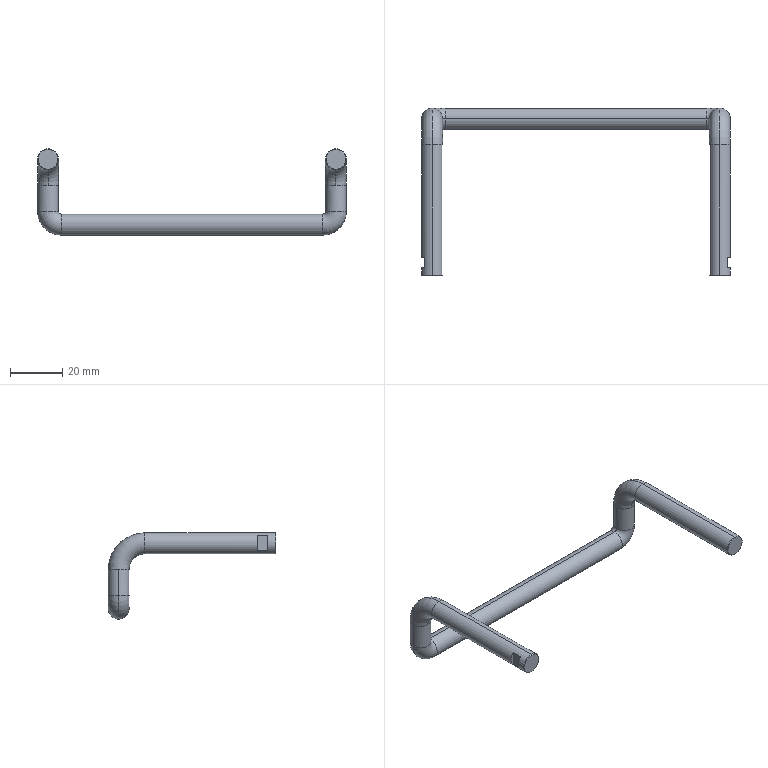Part | SolidWorks | features BaseBody 1 | 1 solid | 30 faces | box 118 x 64 x 33 mm | volume 13386 mm3 | cylinder 10 | torus 8 | plane 8 | cone 4 | commonest cylinder face diameters 8 x10
STEP:
#1=CARTESIAN_POINT('',(-55.,4.,15.));
#2=VERTEX_POINT('',#1);
#3=CARTESIAN_POINT('',(-51.,0.,15.));
#4=VERTEX_POINT('',#3);
#5=CARTESIAN_POINT('',(-55.,0.,15.));
#6=DIRECTION('',(0.,0.,-1.));
#7=DIRECTION('',(0.,-1.,0.));
#8=AXIS2_PLACEMENT_3D('',#5,#6,#7);
#9=CIRCLE('',#8,4.);
#10=EDGE_CURVE('',#2,#4,#9,.T.);
#11=ORIENTED_EDGE('',*,*,#10,.F.);
#12=CARTESIAN_POINT('',(-55.,-10.,29.));
#13=VERTEX_POINT('',#12);
#14=CARTESIAN_POINT('',(-55.,-10.,15.));
#15=DIRECTION('',(1.,0.,0.));
#16=DIRECTION('',(0.,0.,-1.));
#17=AXIS2_PLACEMENT_3D('',#14,#15,#16);
#18=CIRCLE('',#17,14.);
#19=EDGE_CURVE('',#2,#13,#18,.T.);
#20=ORIENTED_EDGE('',*,*,#19,.T.);
#21=CARTESIAN_POINT('',(-55.,-10.,21.));
#22=VERTEX_POINT('',#21);
#23=CARTESIAN_POINT('',(-55.,-10.,25.));
#24=DIRECTION('',(0.,1.,0.));
#25=DIRECTION('',(0.,0.,-1.));
#26=AXIS2_PLACEMENT_3D('',#23,#24,#25);
#27=CIRCLE('',#26,4.);
#28=EDGE_CURVE('',#13,#22,#27,.T.);
#29=ORIENTED_EDGE('',*,*,#28,.T.);
#30=CARTESIAN_POINT('',(-55.,-4.,15.));
#31=VERTEX_POINT('',#30);
#32=CARTESIAN_POINT('',(-55.,-10.,15.));
#33=DIRECTION('',(1.,0.,0.));
#34=DIRECTION('',(0.,0.,-1.));
#35=AXIS2_PLACEMENT_3D('',#32,#33,#34);
#36=CIRCLE('',#35,6.);
#37=EDGE_CURVE('',#31,#22,#36,.T.);
#38=ORIENTED_EDGE('',*,*,#37,.F.);
#39=CARTESIAN_POINT('',(-55.,0.,15.));
#40=DIRECTION('',(0.,0.,-1.));
#41=DIRECTION('',(0.,-1.,0.));
#42=AXIS2_PLACEMENT_3D('',#39,#40,#41);
#43=CIRCLE('',#42,4.);
#44=EDGE_CURVE('',#4,#31,#43,.T.);
#45=ORIENTED_EDGE('',*,*,#44,.F.);
#46=EDGE_LOOP('',(#11,#20,#29,#38,#45));
#47=FACE_OUTER_BOUND('',#46,.T.);
#48=CARTESIAN_POINT('',(-55.,-10.,15.));
#49=DIRECTION('',(1.,0.,0.));
#50=DIRECTION('',(0.,0.,-1.));
#51=AXIS2_PLACEMENT_3D('',#48,#49,#50);
#52=TOROIDAL_SURFACE('',#51,10.,4.);
#53=ADVANCED_FACE('',(#47),#52,.T.);
#54=CARTESIAN_POINT('',(-50.,0.,-4.));
#55=VERTEX_POINT('',#54);
#56=CARTESIAN_POINT('',(-50.,0.,4.));
#57=VERTEX_POINT('',#56);
#58=CARTESIAN_POINT('',(-50.,0.,0.));
#59=DIRECTION('',(1.,0.,0.));
#60=DIRECTION('',(0.,-1.,0.));
#61=AXIS2_PLACEMENT_3D('',#58,#59,#60);
#62=CIRCLE('',#61,4.);
#63=EDGE_CURVE('',#55,#57,#62,.T.);
#64=ORIENTED_EDGE('',*,*,#63,.F.);
#65=CARTESIAN_POINT('',(-59.,0.,5.));
#66=VERTEX_POINT('',#65);
#67=CARTESIAN_POINT('',(-50.,0.,5.));
#68=DIRECTION('',(0.,1.,0.));
#69=DIRECTION('',(0.,0.,1.));
#70=AXIS2_PLACEMENT_3D('',#67,#68,#69);
#71=CIRCLE('',#70,9.);
#72=EDGE_CURVE('',#55,#66,#71,.T.);
#73=ORIENTED_EDGE('',*,*,#72,.T.);
#74=CARTESIAN_POINT('',(-51.,0.,5.));
#75=VERTEX_POINT('',#74);
#76=CARTESIAN_POINT('',(-55.,0.,5.));
#77=DIRECTION('',(0.,0.,-1.));
#78=DIRECTION('',(0.,-1.,0.));
#79=AXIS2_PLACEMENT_3D('',#76,#77,#78);
#80=CIRCLE('',#79,4.);
#81=EDGE_CURVE('',#66,#75,#80,.T.);
#82=ORIENTED_EDGE('',*,*,#81,.T.);
#83=CARTESIAN_POINT('',(-50.,0.,5.));
#84=DIRECTION('',(0.,1.,0.));
#85=DIRECTION('',(0.,0.,1.));
#86=AXIS2_PLACEMENT_3D('',#83,#84,#85);
#87=CIRCLE('',#86,1.);
#88=EDGE_CURVE('',#57,#75,#87,.T.);
#89=ORIENTED_EDGE('',*,*,#88,.F.);
#90=EDGE_LOOP('',(#64,#73,#82,#89));
#91=FACE_OUTER_BOUND('',#90,.T.);
#92=CARTESIAN_POINT('',(-50.,0.,5.));
#93=DIRECTION('',(0.,1.,0.));
#94=DIRECTION('',(0.,0.,1.));
#95=AXIS2_PLACEMENT_3D('',#92,#93,#94);
#96=TOROIDAL_SURFACE('',#95,5.,4.);
#97=ADVANCED_FACE('',(#91),#96,.T.);
#98=CARTESIAN_POINT('',(59.,0.,5.));
#99=VERTEX_POINT('',#98);
#100=CARTESIAN_POINT('',(51.,0.,5.));
#101=VERTEX_POINT('',#100);
#102=CARTESIAN_POINT('',(55.,0.,5.));
#103=DIRECTION('',(0.,0.,1.));
#104=DIRECTION('',(0.,-1.,0.));
#105=AXIS2_PLACEMENT_3D('',#102,#103,#104);
#106=CIRCLE('',#105,4.);
#107=EDGE_CURVE('',#99,#101,#106,.T.);
#108=ORIENTED_EDGE('',*,*,#107,.F.);
#109=CARTESIAN_POINT('',(50.,0.,-4.));
#110=VERTEX_POINT('',#109);
#111=CARTESIAN_POINT('',(50.,0.,5.));
#112=DIRECTION('',(0.,1.,0.));
#113=DIRECTION('',(0.,0.,1.));
#114=AXIS2_PLACEMENT_3D('',#111,#112,#113);
#115=CIRCLE('',#114,9.);
#116=EDGE_CURVE('',#99,#110,#115,.T.);
#117=ORIENTED_EDGE('',*,*,#116,.T.);
#118=CARTESIAN_POINT('',(50.,0.,4.));
#119=VERTEX_POINT('',#118);
#120=CARTESIAN_POINT('',(50.,0.,0.));
#121=DIRECTION('',(1.,0.,0.));
#122=DIRECTION('',(0.,-1.,0.));
#123=AXIS2_PLACEMENT_3D('',#120,#121,#122);
#124=CIRCLE('',#123,4.);
#125=EDGE_CURVE('',#110,#119,#124,.T.);
#126=ORIENTED_EDGE('',*,*,#125,.T.);
#127=CARTESIAN_POINT('',(50.,0.,5.));
#128=DIRECTION('',(0.,1.,0.));
#129=DIRECTION('',(0.,0.,1.));
#130=AXIS2_PLACEMENT_3D('',#127,#128,#129);
#131=CIRCLE('',#130,1.);
#132=EDGE_CURVE('',#101,#119,#131,.T.);
#133=ORIENTED_EDGE('',*,*,#132,.F.);
#134=EDGE_LOOP('',(#108,#117,#126,#133));
#135=FACE_OUTER_BOUND('',#134,.T.);
#136=CARTESIAN_POINT('',(50.,0.,5.));
#137=DIRECTION('',(0.,1.,0.));
#138=DIRECTION('',(0.,0.,1.));
#139=AXIS2_PLACEMENT_3D('',#136,#137,#138);
#140=TOROIDAL_SURFACE('',#139,5.,4.);
#141=ADVANCED_FACE('',(#135),#140,.T.);
#142=CARTESIAN_POINT('',(55.,-10.,29.));
#143=VERTEX_POINT('',#142);
#144=CARTESIAN_POINT('',(55.,-10.,21.));
#145=VERTEX_POINT('',#144);
#146=CARTESIAN_POINT('',(55.,-10.,25.));
#147=DIRECTION('',(0.,-1.,0.));
#148=DIRECTION('',(0.,0.,-1.));
#149=AXIS2_PLACEMENT_3D('',#146,#147,#148);
#150=CIRCLE('',#149,4.);
#151=EDGE_CURVE('',#143,#145,#150,.T.);
#152=ORIENTED_EDGE('',*,*,#151,.F.);
#153=CARTESIAN_POINT('',(55.,4.,15.));
#154=VERTEX_POINT('',#153);
#155=CARTESIAN_POINT('',(55.,-10.,15.));
#156=DIRECTION('',(-1.,0.,0.));
#157=DIRECTION('',(0.,0.,1.));
#158=AXIS2_PLACEMENT_3D('',#155,#156,#157);
#159=CIRCLE('',#158,14.);
#160=EDGE_CURVE('',#143,#154,#159,.T.);
#161=ORIENTED_EDGE('',*,*,#160,.T.);
#162=CARTESIAN_POINT('',(51.,0.,15.));
#163=VERTEX_POINT('',#162);
#164=CARTESIAN_POINT('',(55.,0.,15.));
#165=DIRECTION('',(0.,0.,1.));
#166=DIRECTION('',(0.,-1.,0.));
#167=AXIS2_PLACEMENT_3D('',#164,#165,#166);
#168=CIRCLE('',#167,4.);
#169=EDGE_CURVE('',#154,#163,#168,.T.);
#170=ORIENTED_EDGE('',*,*,#169,.T.);
#171=CARTESIAN_POINT('',(55.,-4.,15.));
#172=VERTEX_POINT('',#171);
#173=CARTESIAN_POINT('',(55.,0.,15.));
#174=DIRECTION('',(0.,0.,1.));
#175=DIRECTION('',(0.,-1.,0.));
#176=AXIS2_PLACEMENT_3D('',#173,#174,#175);
#177=CIRCLE('',#176,4.);
#178=EDGE_CURVE('',#163,#172,#177,.T.);
#179=ORIENTED_EDGE('',*,*,#178,.T.);
#180=CARTESIAN_POINT('',(55.,-10.,15.));
#181=DIRECTION('',(-1.,0.,0.));
#182=DIRECTION('',(0.,0.,1.));
#183=AXIS2_PLACEMENT_3D('',#180,#181,#182);
#184=CIRCLE('',#183,6.);
#185=EDGE_CURVE('',#145,#172,#184,.T.);
#186=ORIENTED_EDGE('',*,*,#185,.F.);
#187=EDGE_LOOP('',(#152,#161,#170,#179,#186));
#188=FACE_OUTER_BOUND('',#187,.T.);
#189=CARTESIAN_POINT('',(55.,-10.,15.));
#190=DIRECTION('',(-1.,0.,0.));
#191=DIRECTION('',(0.,0.,1.));
#192=AXIS2_PLACEMENT_3D('',#189,#190,#191);
#193=TOROIDAL_SURFACE('',#192,10.,4.);
#194=ADVANCED_FACE('',(#188),#193,.T.);
#195=CARTESIAN_POINT('',(-55.,-60.,21.2));
#196=VERTEX_POINT('',#195);
#197=CARTESIAN_POINT('',(-55.,-60.,28.8));
#198=VERTEX_POINT('',#197);
#199=CARTESIAN_POINT('',(-55.,-60.,25.));
#200=DIRECTION('',(0.,-1.,0.));
#201=DIRECTION('',(0.,0.,1.));
#202=AXIS2_PLACEMENT_3D('',#199,#200,#201);
#203=CIRCLE('',#202,3.8);
#204=EDGE_CURVE('',#196,#198,#203,.T.);
#205=ORIENTED_EDGE('',*,*,#204,.F.);
#206=CARTESIAN_POINT('',(-55.,-59.8,21.));
#207=VERTEX_POINT('',#206);
#208=CARTESIAN_POINT('',(-55.,-59.8,21.));
#209=DIRECTION('',(0.,0.7071,-0.7071));
#210=VECTOR('',#209,1000.);
#211=LINE('',#208,#210);
#212=EDGE_CURVE('',#196,#207,#211,.T.);
#213=ORIENTED_EDGE('',*,*,#212,.T.);
#214=CARTESIAN_POINT('',(-55.,-59.8,29.));
#215=VERTEX_POINT('',#214);
#216=CARTESIAN_POINT('',(-55.,-59.8,25.));
#217=DIRECTION('',(0.,1.,0.));
#218=DIRECTION('',(0.,0.,1.));
#219=AXIS2_PLACEMENT_3D('',#216,#217,#218);
#220=CIRCLE('',#219,4.);
#221=EDGE_CURVE('',#215,#207,#220,.T.);
#222=ORIENTED_EDGE('',*,*,#221,.F.);
#223=CARTESIAN_POINT('',(-55.,-59.8,29.));
#224=DIRECTION('',(0.,0.7071,0.7071));
#225=VECTOR('',#224,1000.);
#226=LINE('',#223,#225);
#227=EDGE_CURVE('',#198,#215,#226,.T.);
#228=ORIENTED_EDGE('',*,*,#227,.F.);
#229=EDGE_LOOP('',(#205,#213,#222,#228));
#230=FACE_OUTER_BOUND('',#229,.T.);
#231=CARTESIAN_POINT('',(-55.,-59.8,25.));
#232=DIRECTION('',(0.,1.,0.));
#233=DIRECTION('',(0.,0.,1.));
#234=AXIS2_PLACEMENT_3D('',#231,#232,#233);
#235=CONICAL_SURFACE('',#234,4.,0.7854);
#236=ADVANCED_FACE('',(#230),#235,.T.);
#237=CARTESIAN_POINT('',(55.,-60.,21.2));
#238=VERTEX_POINT('',#237);
#239=CARTESIAN_POINT('',(55.,-60.,28.8));
#240=VERTEX_POINT('',#239);
#241=CARTESIAN_POINT('',(55.,-60.,25.));
#242=DIRECTION('',(0.,-1.,0.));
#243=DIRECTION('',(0.,0.,-1.));
#244=AXIS2_PLACEMENT_3D('',#241,#242,#243);
#245=CIRCLE('',#244,3.8);
#246=EDGE_CURVE('',#238,#240,#245,.T.);
#247=ORIENTED_EDGE('',*,*,#246,.F.);
#248=CARTESIAN_POINT('',(55.,-59.8,21.));
#249=VERTEX_POINT('',#248);
#250=CARTESIAN_POINT('',(55.,-60.,21.2));
#251=DIRECTION('',(0.,0.7071,-0.7071));
#252=VECTOR('',#251,1000.);
#253=LINE('',#250,#252);
#254=EDGE_CURVE('',#238,#249,#253,.T.);
#255=ORIENTED_EDGE('',*,*,#254,.T.);
#256=CARTESIAN_POINT('',(55.,-59.8,29.));
#257=VERTEX_POINT('',#256);
#258=CARTESIAN_POINT('',(55.,-59.8,25.));
#259=DIRECTION('',(0.,1.,0.));
#260=DIRECTION('',(0.,0.,-1.));
#261=AXIS2_PLACEMENT_3D('',#258,#259,#260);
#262=CIRCLE('',#261,4.);
#263=EDGE_CURVE('',#257,#249,#262,.T.);
#264=ORIENTED_EDGE('',*,*,#263,.F.);
#265=CARTESIAN_POINT('',(55.,-60.,28.8));
#266=DIRECTION('',(0.,0.7071,0.7071));
#267=VECTOR('',#266,1000.);
#268=LINE('',#265,#267);
#269=EDGE_CURVE('',#240,#257,#268,.T.);
#270=ORIENTED_EDGE('',*,*,#269,.F.);
#271=EDGE_LOOP('',(#247,#255,#264,#270));
#272=FACE_OUTER_BOUND('',#271,.T.);
#273=CARTESIAN_POINT('',(55.,-60.,25.));
#274=DIRECTION('',(0.,1.,0.));
#275=DIRECTION('',(0.,0.,1.));
#276=AXIS2_PLACEMENT_3D('',#273,#274,#275);
#277=CONICAL_SURFACE('',#276,3.8,0.7854);
#278=ADVANCED_FACE('',(#272),#277,.T.);
#279=ORIENTED_EDGE('',*,*,#28,.F.);
#280=CARTESIAN_POINT('',(-55.,-10.,29.));
#281=DIRECTION('',(0.,-1.,0.));
#282=VECTOR('',#281,1000.);
#283=LINE('',#280,#282);
#284=EDGE_CURVE('',#13,#215,#283,.T.);
#285=ORIENTED_EDGE('',*,*,#284,.T.);
#286=ORIENTED_EDGE('',*,*,#221,.T.);
#287=CARTESIAN_POINT('',(-55.,-10.,21.));
#288=DIRECTION('',(0.,-1.,0.));
#289=VECTOR('',#288,1000.);
#290=LINE('',#287,#289);
#291=EDGE_CURVE('',#22,#207,#290,.T.);
#292=ORIENTED_EDGE('',*,*,#291,.F.);
#293=EDGE_LOOP('',(#279,#285,#286,#292));
#294=FACE_OUTER_BOUND('',#293,.T.);
#295=CARTESIAN_POINT('',(-55.,-10.,25.));
#296=DIRECTION('',(0.,-1.,0.));
#297=DIRECTION('',(0.,0.,-1.));
#298=AXIS2_PLACEMENT_3D('',#295,#296,#297);
#299=CYLINDRICAL_SURFACE('',#298,4.);
#300=ADVANCED_FACE('',(#294),#299,.T.);
#301=ORIENTED_EDGE('',*,*,#81,.F.);
#302=CARTESIAN_POINT('',(-59.,0.,15.));
#303=VERTEX_POINT('',#302);
#304=CARTESIAN_POINT('',(-59.,0.,5.));
#305=DIRECTION('',(0.,0.,1.));
#306=VECTOR('',#305,1000.);
#307=LINE('',#304,#306);
#308=EDGE_CURVE('',#66,#303,#307,.T.);
#309=ORIENTED_EDGE('',*,*,#308,.T.);
#310=CARTESIAN_POINT('',(-55.,0.,15.));
#311=DIRECTION('',(0.,0.,-1.));
#312=DIRECTION('',(0.,-1.,0.));
#313=AXIS2_PLACEMENT_3D('',#310,#311,#312);
#314=CIRCLE('',#313,4.);
#315=EDGE_CURVE('',#303,#2,#314,.T.);
#316=ORIENTED_EDGE('',*,*,#315,.T.);
#317=ORIENTED_EDGE('',*,*,#10,.T.);
#318=CARTESIAN_POINT('',(-51.,0.,5.));
#319=DIRECTION('',(0.,0.,1.));
#320=VECTOR('',#319,1000.);
#321=LINE('',#318,#320);
#322=EDGE_CURVE('',#75,#4,#321,.T.);
#323=ORIENTED_EDGE('',*,*,#322,.F.);
#324=EDGE_LOOP('',(#301,#309,#316,#317,#323));
#325=FACE_OUTER_BOUND('',#324,.T.);
#326=CARTESIAN_POINT('',(-55.,0.,5.));
#327=DIRECTION('',(0.,0.,1.));
#328=DIRECTION('',(1.,0.,0.));
#329=AXIS2_PLACEMENT_3D('',#326,#327,#328);
#330=CYLINDRICAL_SURFACE('',#329,4.);
#331=ADVANCED_FACE('',(#325),#330,.T.);
#332=ORIENTED_EDGE('',*,*,#125,.F.);
#333=CARTESIAN_POINT('',(50.,0.,-4.));
#334=DIRECTION('',(-1.,0.,0.));
#335=VECTOR('',#334,1000.);
#336=LINE('',#333,#335);
#337=EDGE_CURVE('',#110,#55,#336,.T.);
#338=ORIENTED_EDGE('',*,*,#337,.T.);
#339=ORIENTED_EDGE('',*,*,#63,.T.);
#340=CARTESIAN_POINT('',(50.,0.,4.));
#341=DIRECTION('',(-1.,0.,0.));
#342=VECTOR('',#341,1000.);
#343=LINE('',#340,#342);
#344=EDGE_CURVE('',#119,#57,#343,.T.);
#345=ORIENTED_EDGE('',*,*,#344,.F.);
#346=EDGE_LOOP('',(#332,#338,#339,#345));
#347=FACE_OUTER_BOUND('',#346,.T.);
#348=CARTESIAN_POINT('',(50.,0.,0.));
#349=DIRECTION('',(-1.,0.,0.));
#350=DIRECTION('',(0.,0.,1.));
#351=AXIS2_PLACEMENT_3D('',#348,#349,#350);
#352=CYLINDRICAL_SURFACE('',#351,4.);
#353=ADVANCED_FACE('',(#347),#352,.T.);
#354=CARTESIAN_POINT('',(59.,0.,15.));
#355=VERTEX_POINT('',#354);
#356=CARTESIAN_POINT('',(55.,0.,15.));
#357=DIRECTION('',(0.,0.,1.));
#358=DIRECTION('',(0.,-1.,0.));
#359=AXIS2_PLACEMENT_3D('',#356,#357,#358);
#360=CIRCLE('',#359,4.);
#361=EDGE_CURVE('',#355,#154,#360,.T.);
#362=ORIENTED_EDGE('',*,*,#361,.F.);
#363=CARTESIAN_POINT('',(59.,0.,15.));
#364=DIRECTION('',(0.,0.,-1.));
#365=VECTOR('',#364,1000.);
#366=LINE('',#363,#365);
#367=EDGE_CURVE('',#355,#99,#366,.T.);
#368=ORIENTED_EDGE('',*,*,#367,.T.);
#369=ORIENTED_EDGE('',*,*,#107,.T.);
#370=CARTESIAN_POINT('',(51.,0.,15.));
#371=DIRECTION('',(0.,0.,-1.));
#372=VECTOR('',#371,1000.);
#373=LINE('',#370,#372);
#374=EDGE_CURVE('',#163,#101,#373,.T.);
#375=ORIENTED_EDGE('',*,*,#374,.F.);
#376=ORIENTED_EDGE('',*,*,#169,.F.);
#377=EDGE_LOOP('',(#362,#368,#369,#375,#376));
#378=FACE_OUTER_BOUND('',#377,.T.);
#379=CARTESIAN_POINT('',(55.,0.,15.));
#380=DIRECTION('',(0.,0.,-1.));
#381=DIRECTION('',(-1.,0.,0.));
#382=AXIS2_PLACEMENT_3D('',#379,#380,#381);
#383=CYLINDRICAL_SURFACE('',#382,4.);
#384=ADVANCED_FACE('',(#378),#383,.T.);
#385=CARTESIAN_POINT('',(57.75,-53.,22.095));
#386=VERTEX_POINT('',#385);
#387=CARTESIAN_POINT('',(57.75,-57.,22.095));
#388=VERTEX_POINT('',#387);
#389=CARTESIAN_POINT('',(57.75,-60.,22.095));
#390=DIRECTION('',(0.,-1.,0.));
#391=VECTOR('',#390,1000.);
#392=LINE('',#389,#391);
#393=EDGE_CURVE('',#386,#388,#392,.T.);
#394=ORIENTED_EDGE('',*,*,#393,.T.);
#395=CARTESIAN_POINT('',(57.75,-57.,27.905));
#396=VERTEX_POINT('',#395);
#397=CARTESIAN_POINT('',(55.,-57.,25.));
#398=DIRECTION('',(0.,-1.,0.));
#399=DIRECTION('',(0.,0.,-1.));
#400=AXIS2_PLACEMENT_3D('',#397,#398,#399);
#401=CIRCLE('',#400,4.);
#402=EDGE_CURVE('',#388,#396,#401,.T.);
#403=ORIENTED_EDGE('',*,*,#402,.T.);
#404=CARTESIAN_POINT('',(57.75,-53.,27.905));
#405=VERTEX_POINT('',#404);
#406=CARTESIAN_POINT('',(57.75,-60.,27.905));
#407=DIRECTION('',(0.,1.,0.));
#408=VECTOR('',#407,1000.);
#409=LINE('',#406,#408);
#410=EDGE_CURVE('',#396,#405,#409,.T.);
#411=ORIENTED_EDGE('',*,*,#410,.T.);
#412=CARTESIAN_POINT('',(55.,-53.,25.));
#413=DIRECTION('',(0.,1.,0.));
#414=DIRECTION('',(0.,0.,1.));
#415=AXIS2_PLACEMENT_3D('',#412,#413,#414);
#416=CIRCLE('',#415,4.);
#417=EDGE_CURVE('',#405,#386,#416,.T.);
#418=ORIENTED_EDGE('',*,*,#417,.T.);
#419=EDGE_LOOP('',(#394,#403,#411,#418));
#420=FACE_BOUND('',#419,.T.);
#421=ORIENTED_EDGE('',*,*,#263,.T.);
#422=CARTESIAN_POINT('',(55.,-60.,21.));
#423=DIRECTION('',(0.,1.,0.));
#424=VECTOR('',#423,1000.);
#425=LINE('',#422,#424);
#426=EDGE_CURVE('',#249,#145,#425,.T.);
#427=ORIENTED_EDGE('',*,*,#426,.T.);
#428=CARTESIAN_POINT('',(55.,-10.,25.));
#429=DIRECTION('',(0.,-1.,0.));
#430=DIRECTION('',(0.,0.,-1.));
#431=AXIS2_PLACEMENT_3D('',#428,#429,#430);
#432=CIRCLE('',#431,4.);
#433=EDGE_CURVE('',#145,#143,#432,.T.);
#434=ORIENTED_EDGE('',*,*,#433,.T.);
#435=CARTESIAN_POINT('',(55.,-60.,29.));
#436=DIRECTION('',(0.,1.,0.));
#437=VECTOR('',#436,1000.);
#438=LINE('',#435,#437);
#439=EDGE_CURVE('',#257,#143,#438,.T.);
#440=ORIENTED_EDGE('',*,*,#439,.F.);
#441=EDGE_LOOP('',(#421,#427,#434,#440));
#442=FACE_OUTER_BOUND('',#441,.T.);
#443=CARTESIAN_POINT('',(55.,-60.,25.));
#444=DIRECTION('',(0.,1.,0.));
#445=DIRECTION('',(0.,0.,1.));
#446=AXIS2_PLACEMENT_3D('',#443,#444,#445);
#447=CYLINDRICAL_SURFACE('',#446,4.);
#448=ADVANCED_FACE('',(#420,#442),#447,.T.);
#449=CARTESIAN_POINT('',(57.75,-53.,-4.));
#450=DIRECTION('',(0.,0.,1.));
#451=VECTOR('',#450,1000.);
#452=LINE('',#449,#451);
#453=EDGE_CURVE('',#386,#405,#452,.T.);
#454=ORIENTED_EDGE('',*,*,#453,.F.);
#455=ORIENTED_EDGE('',*,*,#417,.F.);
#456=EDGE_LOOP('',(#454,#455));
#457=FACE_OUTER_BOUND('',#456,.T.);
#458=CARTESIAN_POINT('',(57.75,-53.,-4.));
#459=DIRECTION('',(0.,1.,0.));
#460=DIRECTION('',(1.,0.,0.));
#461=AXIS2_PLACEMENT_3D('',#458,#459,#460);
#462=PLANE('',#461);
#463=ADVANCED_FACE('',(#457),#462,.F.);
#464=CARTESIAN_POINT('',(57.75,-57.,-4.));
#465=DIRECTION('',(0.,0.,1.));
#466=VECTOR('',#465,1000.);
#467=LINE('',#464,#466);
#468=EDGE_CURVE('',#388,#396,#467,.T.);
#469=ORIENTED_EDGE('',*,*,#468,.F.);
#470=ORIENTED_EDGE('',*,*,#393,.F.);
#471=ORIENTED_EDGE('',*,*,#453,.T.);
#472=ORIENTED_EDGE('',*,*,#410,.F.);
#473=EDGE_LOOP('',(#469,#470,#471,#472));
#474=FACE_OUTER_BOUND('',#473,.T.);
#475=CARTESIAN_POINT('',(57.75,-57.,-4.));
#476=DIRECTION('',(-1.,0.,0.));
#477=DIRECTION('',(0.,1.,0.));
#478=AXIS2_PLACEMENT_3D('',#475,#476,#477);
#479=PLANE('',#478);
#480=ADVANCED_FACE('',(#474),#479,.F.);
#481=ORIENTED_EDGE('',*,*,#468,.T.);
#482=ORIENTED_EDGE('',*,*,#402,.F.);
#483=EDGE_LOOP('',(#481,#482));
#484=FACE_OUTER_BOUND('',#483,.T.);
#485=CARTESIAN_POINT('',(57.75,-57.,-4.));
#486=DIRECTION('',(0.,-1.,0.));
#487=DIRECTION('',(0.,0.,-1.));
#488=AXIS2_PLACEMENT_3D('',#485,#486,#487);
#489=PLANE('',#488);
#490=ADVANCED_FACE('',(#484),#489,.F.);
#491=CARTESIAN_POINT('',(-57.75,-53.,22.095));
#492=VERTEX_POINT('',#491);
#493=CARTESIAN_POINT('',(-57.75,-53.,27.905));
#494=VERTEX_POINT('',#493);
#495=CARTESIAN_POINT('',(-57.75,-53.,-4.));
#496=DIRECTION('',(0.,0.,1.));
#497=VECTOR('',#496,1000.);
#498=LINE('',#495,#497);
#499=EDGE_CURVE('',#492,#494,#498,.T.);
#500=ORIENTED_EDGE('',*,*,#499,.T.);
#501=CARTESIAN_POINT('',(-55.,-53.,25.));
#502=DIRECTION('',(0.,1.,0.));
#503=DIRECTION('',(-1.,0.,0.));
#504=AXIS2_PLACEMENT_3D('',#501,#502,#503);
#505=CIRCLE('',#504,4.);
#506=EDGE_CURVE('',#492,#494,#505,.T.);
#507=ORIENTED_EDGE('',*,*,#506,.F.);
#508=EDGE_LOOP('',(#500,#507));
#509=FACE_OUTER_BOUND('',#508,.T.);
#510=CARTESIAN_POINT('',(-60.25,-53.,-4.));
#511=DIRECTION('',(0.,1.,0.));
#512=DIRECTION('',(1.,0.,0.));
#513=AXIS2_PLACEMENT_3D('',#510,#511,#512);
#514=PLANE('',#513);
#515=ADVANCED_FACE('',(#509),#514,.F.);
#516=CARTESIAN_POINT('',(-57.75,-57.,22.095));
#517=VERTEX_POINT('',#516);
#518=CARTESIAN_POINT('',(-57.75,-57.,27.905));
#519=VERTEX_POINT('',#518);
#520=CARTESIAN_POINT('',(-57.75,-57.,-4.));
#521=DIRECTION('',(0.,0.,1.));
#522=VECTOR('',#521,1000.);
#523=LINE('',#520,#522);
#524=EDGE_CURVE('',#517,#519,#523,.T.);
#525=ORIENTED_EDGE('',*,*,#524,.F.);
#526=CARTESIAN_POINT('',(-55.,-57.,25.));
#527=DIRECTION('',(0.,-1.,0.));
#528=DIRECTION('',(0.,0.,-1.));
#529=AXIS2_PLACEMENT_3D('',#526,#527,#528);
#530=CIRCLE('',#529,4.);
#531=EDGE_CURVE('',#519,#517,#530,.T.);
#532=ORIENTED_EDGE('',*,*,#531,.F.);
#533=EDGE_LOOP('',(#525,#532));
#534=FACE_OUTER_BOUND('',#533,.T.);
#535=CARTESIAN_POINT('',(-60.25,-57.,-4.));
#536=DIRECTION('',(0.,-1.,0.));
#537=DIRECTION('',(0.,0.,-1.));
#538=AXIS2_PLACEMENT_3D('',#535,#536,#537);
#539=PLANE('',#538);
#540=ADVANCED_FACE('',(#534),#539,.F.);
#541=ORIENTED_EDGE('',*,*,#499,.F.);
#542=CARTESIAN_POINT('',(-57.75,-10.,22.095));
#543=DIRECTION('',(0.,1.,0.));
#544=VECTOR('',#543,1000.);
#545=LINE('',#542,#544);
#546=EDGE_CURVE('',#517,#492,#545,.T.);
#547=ORIENTED_EDGE('',*,*,#546,.F.);
#548=ORIENTED_EDGE('',*,*,#524,.T.);
#549=CARTESIAN_POINT('',(-57.75,-10.,27.905));
#550=DIRECTION('',(0.,-1.,0.));
#551=VECTOR('',#550,1000.);
#552=LINE('',#549,#551);
#553=EDGE_CURVE('',#494,#519,#552,.T.);
#554=ORIENTED_EDGE('',*,*,#553,.F.);
#555=EDGE_LOOP('',(#541,#547,#548,#554));
#556=FACE_OUTER_BOUND('',#555,.T.);
#557=CARTESIAN_POINT('',(-57.75,-57.,-4.));
#558=DIRECTION('',(1.,0.,0.));
#559=DIRECTION('',(0.,1.,0.));
#560=AXIS2_PLACEMENT_3D('',#557,#558,#559);
#561=PLANE('',#560);
#562=ADVANCED_FACE('',(#556),#561,.F.);
#563=CARTESIAN_POINT('',(55.,-60.,25.));
#564=DIRECTION('',(0.,-1.,0.));
#565=DIRECTION('',(0.,0.,-1.));
#566=AXIS2_PLACEMENT_3D('',#563,#564,#565);
#567=CIRCLE('',#566,3.8);
#568=EDGE_CURVE('',#240,#238,#567,.T.);
#569=ORIENTED_EDGE('',*,*,#568,.T.);
#570=ORIENTED_EDGE('',*,*,#246,.T.);
#571=EDGE_LOOP('',(#569,#570));
#572=FACE_OUTER_BOUND('',#571,.T.);
#573=CARTESIAN_POINT('',(55.,-60.,25.));
#574=DIRECTION('',(0.,-1.,0.));
#575=DIRECTION('',(0.,0.,-1.));
#576=AXIS2_PLACEMENT_3D('',#573,#574,#575);
#577=PLANE('',#576);
#578=ADVANCED_FACE('',(#572),#577,.T.);
#579=CARTESIAN_POINT('',(-55.,-60.,25.));
#580=DIRECTION('',(0.,-1.,0.));
#581=DIRECTION('',(0.,0.,1.));
#582=AXIS2_PLACEMENT_3D('',#579,#580,#581);
#583=CIRCLE('',#582,3.8);
#584=EDGE_CURVE('',#198,#196,#583,.T.);
#585=ORIENTED_EDGE('',*,*,#584,.T.);
#586=ORIENTED_EDGE('',*,*,#204,.T.);
#587=EDGE_LOOP('',(#585,#586));
#588=FACE_OUTER_BOUND('',#587,.T.);
#589=CARTESIAN_POINT('',(-55.,-60.,25.));
#590=DIRECTION('',(0.,1.,0.));
#591=DIRECTION('',(1.,0.,0.));
#592=AXIS2_PLACEMENT_3D('',#589,#590,#591);
#593=PLANE('',#592);
#594=ADVANCED_FACE('',(#588),#593,.F.);
#595=ORIENTED_EDGE('',*,*,#426,.F.);
#596=CARTESIAN_POINT('',(55.,-59.8,25.));
#597=DIRECTION('',(0.,1.,0.));
#598=DIRECTION('',(0.,0.,-1.));
#599=AXIS2_PLACEMENT_3D('',#596,#597,#598);
#600=CIRCLE('',#599,4.);
#601=EDGE_CURVE('',#249,#257,#600,.T.);
#602=ORIENTED_EDGE('',*,*,#601,.T.);
#603=ORIENTED_EDGE('',*,*,#439,.T.);
#604=ORIENTED_EDGE('',*,*,#151,.T.);
#605=EDGE_LOOP('',(#595,#602,#603,#604));
#606=FACE_OUTER_BOUND('',#605,.T.);
#607=CARTESIAN_POINT('',(55.,-60.,25.));
#608=DIRECTION('',(0.,1.,0.));
#609=DIRECTION('',(0.,0.,1.));
#610=AXIS2_PLACEMENT_3D('',#607,#608,#609);
#611=CYLINDRICAL_SURFACE('',#610,4.);
#612=ADVANCED_FACE('',(#606),#611,.T.);
#613=ORIENTED_EDGE('',*,*,#367,.F.);
#614=CARTESIAN_POINT('',(55.,0.,15.));
#615=DIRECTION('',(0.,0.,1.));
#616=DIRECTION('',(0.,-1.,0.));
#617=AXIS2_PLACEMENT_3D('',#614,#615,#616);
#618=CIRCLE('',#617,4.);
#619=EDGE_CURVE('',#172,#355,#618,.T.);
#620=ORIENTED_EDGE('',*,*,#619,.F.);
#621=ORIENTED_EDGE('',*,*,#178,.F.);
#622=ORIENTED_EDGE('',*,*,#374,.T.);
#623=CARTESIAN_POINT('',(55.,0.,5.));
#624=DIRECTION('',(0.,0.,1.));
#625=DIRECTION('',(0.,-1.,0.));
#626=AXIS2_PLACEMENT_3D('',#623,#624,#625);
#627=CIRCLE('',#626,4.);
#628=EDGE_CURVE('',#101,#99,#627,.T.);
#629=ORIENTED_EDGE('',*,*,#628,.T.);
#630=EDGE_LOOP('',(#613,#620,#621,#622,#629));
#631=FACE_OUTER_BOUND('',#630,.T.);
#632=CARTESIAN_POINT('',(55.,0.,15.));
#633=DIRECTION('',(0.,0.,-1.));
#634=DIRECTION('',(-1.,0.,0.));
#635=AXIS2_PLACEMENT_3D('',#632,#633,#634);
#636=CYLINDRICAL_SURFACE('',#635,4.);
#637=ADVANCED_FACE('',(#631),#636,.T.);
#638=ORIENTED_EDGE('',*,*,#337,.F.);
#639=CARTESIAN_POINT('',(50.,0.,0.));
#640=DIRECTION('',(1.,0.,0.));
#641=DIRECTION('',(0.,-1.,0.));
#642=AXIS2_PLACEMENT_3D('',#639,#640,#641);
#643=CIRCLE('',#642,4.);
#644=EDGE_CURVE('',#119,#110,#643,.T.);
#645=ORIENTED_EDGE('',*,*,#644,.F.);
#646=ORIENTED_EDGE('',*,*,#344,.T.);
#647=CARTESIAN_POINT('',(-50.,0.,0.));
#648=DIRECTION('',(1.,0.,0.));
#649=DIRECTION('',(0.,-1.,0.));
#650=AXIS2_PLACEMENT_3D('',#647,#648,#649);
#651=CIRCLE('',#650,4.);
#652=EDGE_CURVE('',#57,#55,#651,.T.);
#653=ORIENTED_EDGE('',*,*,#652,.T.);
#654=EDGE_LOOP('',(#638,#645,#646,#653));
#655=FACE_OUTER_BOUND('',#654,.T.);
#656=CARTESIAN_POINT('',(50.,0.,0.));
#657=DIRECTION('',(-1.,0.,0.));
#658=DIRECTION('',(0.,0.,1.));
#659=AXIS2_PLACEMENT_3D('',#656,#657,#658);
#660=CYLINDRICAL_SURFACE('',#659,4.);
#661=ADVANCED_FACE('',(#655),#660,.T.);
#662=ORIENTED_EDGE('',*,*,#308,.F.);
#663=CARTESIAN_POINT('',(-55.,0.,5.));
#664=DIRECTION('',(0.,0.,-1.));
#665=DIRECTION('',(0.,-1.,0.));
#666=AXIS2_PLACEMENT_3D('',#663,#664,#665);
#667=CIRCLE('',#666,4.);
#668=EDGE_CURVE('',#75,#66,#667,.T.);
#669=ORIENTED_EDGE('',*,*,#668,.F.);
#670=ORIENTED_EDGE('',*,*,#322,.T.);
#671=ORIENTED_EDGE('',*,*,#44,.T.);
#672=CARTESIAN_POINT('',(-55.,0.,15.));
#673=DIRECTION('',(0.,0.,-1.));
#674=DIRECTION('',(0.,-1.,0.));
#675=AXIS2_PLACEMENT_3D('',#672,#673,#674);
#676=CIRCLE('',#675,4.);
#677=EDGE_CURVE('',#31,#303,#676,.T.);
#678=ORIENTED_EDGE('',*,*,#677,.T.);
#679=EDGE_LOOP('',(#662,#669,#670,#671,#678));
#680=FACE_OUTER_BOUND('',#679,.T.);
#681=CARTESIAN_POINT('',(-55.,0.,5.));
#682=DIRECTION('',(0.,0.,1.));
#683=DIRECTION('',(1.,0.,0.));
#684=AXIS2_PLACEMENT_3D('',#681,#682,#683);
#685=CYLINDRICAL_SURFACE('',#684,4.);
#686=ADVANCED_FACE('',(#680),#685,.T.);
#687=ORIENTED_EDGE('',*,*,#284,.F.);
#688=CARTESIAN_POINT('',(-55.,-10.,25.));
#689=DIRECTION('',(0.,1.,0.));
#690=DIRECTION('',(0.,0.,-1.));
#691=AXIS2_PLACEMENT_3D('',#688,#689,#690);
#692=CIRCLE('',#691,4.);
#693=EDGE_CURVE('',#22,#13,#692,.T.);
#694=ORIENTED_EDGE('',*,*,#693,.F.);
#695=ORIENTED_EDGE('',*,*,#291,.T.);
#696=CARTESIAN_POINT('',(-55.,-59.8,25.));
#697=DIRECTION('',(0.,1.,0.));
#698=DIRECTION('',(0.,0.,1.));
#699=AXIS2_PLACEMENT_3D('',#696,#697,#698);
#700=CIRCLE('',#699,4.);
#701=EDGE_CURVE('',#207,#215,#700,.T.);
#702=ORIENTED_EDGE('',*,*,#701,.T.);
#703=EDGE_LOOP('',(#687,#694,#695,#702));
#704=FACE_OUTER_BOUND('',#703,.T.);
#705=ORIENTED_EDGE('',*,*,#553,.T.);
#706=ORIENTED_EDGE('',*,*,#531,.T.);
#707=ORIENTED_EDGE('',*,*,#546,.T.);
#708=ORIENTED_EDGE('',*,*,#506,.T.);
#709=EDGE_LOOP('',(#705,#706,#707,#708));
#710=FACE_BOUND('',#709,.T.);
#711=CARTESIAN_POINT('',(-55.,-10.,25.));
#712=DIRECTION('',(0.,-1.,0.));
#713=DIRECTION('',(0.,0.,-1.));
#714=AXIS2_PLACEMENT_3D('',#711,#712,#713);
#715=CYLINDRICAL_SURFACE('',#714,4.);
#716=ADVANCED_FACE('',(#704,#710),#715,.T.);
#717=ORIENTED_EDGE('',*,*,#254,.F.);
#718=ORIENTED_EDGE('',*,*,#568,.F.);
#719=ORIENTED_EDGE('',*,*,#269,.T.);
#720=ORIENTED_EDGE('',*,*,#601,.F.);
#721=EDGE_LOOP('',(#717,#718,#719,#720));
#722=FACE_OUTER_BOUND('',#721,.T.);
#723=CARTESIAN_POINT('',(55.,-60.,25.));
#724=DIRECTION('',(0.,1.,0.));
#725=DIRECTION('',(0.,0.,1.));
#726=AXIS2_PLACEMENT_3D('',#723,#724,#725);
#727=CONICAL_SURFACE('',#726,3.8,0.7854);
#728=ADVANCED_FACE('',(#722),#727,.T.);
#729=ORIENTED_EDGE('',*,*,#212,.F.);
#730=ORIENTED_EDGE('',*,*,#584,.F.);
#731=ORIENTED_EDGE('',*,*,#227,.T.);
#732=ORIENTED_EDGE('',*,*,#701,.F.);
#733=EDGE_LOOP('',(#729,#730,#731,#732));
#734=FACE_OUTER_BOUND('',#733,.T.);
#735=CARTESIAN_POINT('',(-55.,-59.8,25.));
#736=DIRECTION('',(0.,1.,0.));
#737=DIRECTION('',(0.,0.,1.));
#738=AXIS2_PLACEMENT_3D('',#735,#736,#737);
#739=CONICAL_SURFACE('',#738,4.,0.7854);
#740=ADVANCED_FACE('',(#734),#739,.T.);
#741=ORIENTED_EDGE('',*,*,#160,.F.);
#742=ORIENTED_EDGE('',*,*,#433,.F.);
#743=ORIENTED_EDGE('',*,*,#185,.T.);
#744=ORIENTED_EDGE('',*,*,#619,.T.);
#745=ORIENTED_EDGE('',*,*,#361,.T.);
#746=EDGE_LOOP('',(#741,#742,#743,#744,#745));
#747=FACE_OUTER_BOUND('',#746,.T.);
#748=CARTESIAN_POINT('',(55.,-10.,15.));
#749=DIRECTION('',(-1.,0.,0.));
#750=DIRECTION('',(0.,0.,1.));
#751=AXIS2_PLACEMENT_3D('',#748,#749,#750);
#752=TOROIDAL_SURFACE('',#751,10.,4.);
#753=ADVANCED_FACE('',(#747),#752,.T.);
#754=ORIENTED_EDGE('',*,*,#116,.F.);
#755=ORIENTED_EDGE('',*,*,#628,.F.);
#756=ORIENTED_EDGE('',*,*,#132,.T.);
#757=ORIENTED_EDGE('',*,*,#644,.T.);
#758=EDGE_LOOP('',(#754,#755,#756,#757));
#759=FACE_OUTER_BOUND('',#758,.T.);
#760=CARTESIAN_POINT('',(50.,0.,5.));
#761=DIRECTION('',(0.,1.,0.));
#762=DIRECTION('',(0.,0.,1.));
#763=AXIS2_PLACEMENT_3D('',#760,#761,#762);
#764=TOROIDAL_SURFACE('',#763,5.,4.);
#765=ADVANCED_FACE('',(#759),#764,.T.);
#766=ORIENTED_EDGE('',*,*,#72,.F.);
#767=ORIENTED_EDGE('',*,*,#652,.F.);
#768=ORIENTED_EDGE('',*,*,#88,.T.);
#769=ORIENTED_EDGE('',*,*,#668,.T.);
#770=EDGE_LOOP('',(#766,#767,#768,#769));
#771=FACE_OUTER_BOUND('',#770,.T.);
#772=CARTESIAN_POINT('',(-50.,0.,5.));
#773=DIRECTION('',(0.,1.,0.));
#774=DIRECTION('',(0.,0.,1.));
#775=AXIS2_PLACEMENT_3D('',#772,#773,#774);
#776=TOROIDAL_SURFACE('',#775,5.,4.);
#777=ADVANCED_FACE('',(#771),#776,.T.);
#778=ORIENTED_EDGE('',*,*,#19,.F.);
#779=ORIENTED_EDGE('',*,*,#315,.F.);
#780=ORIENTED_EDGE('',*,*,#677,.F.);
#781=ORIENTED_EDGE('',*,*,#37,.T.);
#782=ORIENTED_EDGE('',*,*,#693,.T.);
#783=EDGE_LOOP('',(#778,#779,#780,#781,#782));
#784=FACE_OUTER_BOUND('',#783,.T.);
#785=CARTESIAN_POINT('',(-55.,-10.,15.));
#786=DIRECTION('',(1.,0.,0.));
#787=DIRECTION('',(0.,0.,-1.));
#788=AXIS2_PLACEMENT_3D('',#785,#786,#787);
#789=TOROIDAL_SURFACE('',#788,10.,4.);
#790=ADVANCED_FACE('',(#784),#789,.T.);
#791=CLOSED_SHELL('',(#53,#97,#141,#194,#236,#278,#300,#331,#353,#384,#448,#463,#480,#490,#515,#540,#562,#578,#594,#612,#637,#661,#686,#716,#728,#740,#753,#765,#777,#790));
#792=MANIFOLD_SOLID_BREP('',#791);
#793=CARTESIAN_POINT('',(0.,0.,0.));
#794=DIRECTION('',(0.,0.,1.));
#795=DIRECTION('',(1.,0.,0.));
#796=AXIS2_PLACEMENT_3D('',#793,#794,#795);
#797=(LENGTH_UNIT()NAMED_UNIT(*)SI_UNIT(.MILLI.,.METRE.));
#798=UNCERTAINTY_MEASURE_WITH_UNIT(LENGTH_MEASURE(0.00001),#797,'','');
#799=(NAMED_UNIT(*)PLANE_ANGLE_UNIT()SI_UNIT($,.RADIAN.));
#800=(NAMED_UNIT(*)SI_UNIT($,.STERADIAN.)SOLID_ANGLE_UNIT());
#801=(GEOMETRIC_REPRESENTATION_CONTEXT(3)GLOBAL_UNCERTAINTY_ASSIGNED_CONTEXT((#798))GLOBAL_UNIT_ASSIGNED_CONTEXT((#797,#799,#800))REPRESENTATION_CONTEXT('',''));
#802=ADVANCED_BREP_SHAPE_REPRESENTATION('',(#792,#796),#801);